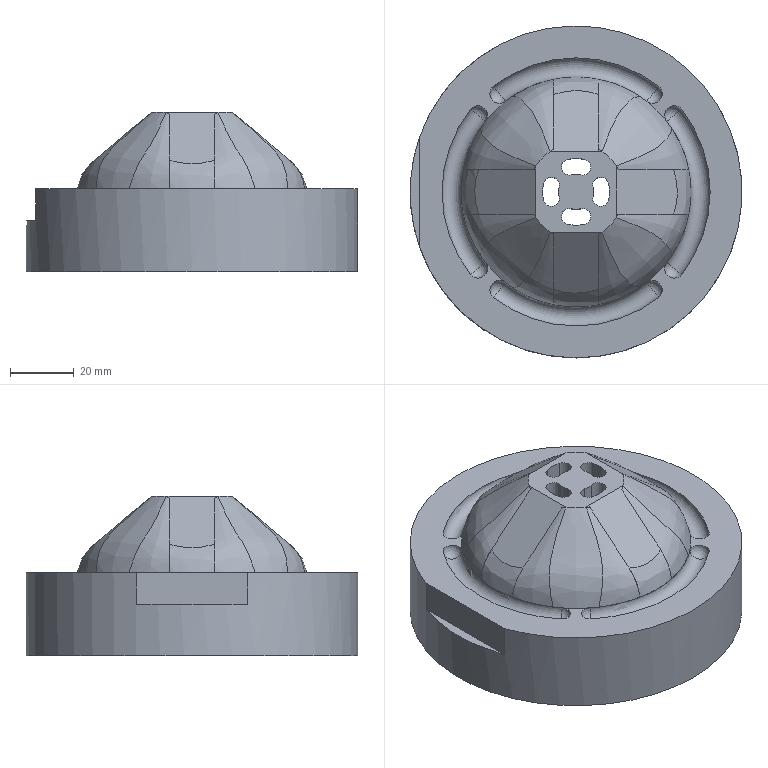Part | 1 solid | 66 faces | box 104 x 104 x 49.86 mm | volume 267956 mm3 | plane 20 | spline 17 | cylinder 17 | sphere 8 | torus 4 | commonest cylinder face diameters 5 x8 11 x4 21 x4 104 x1